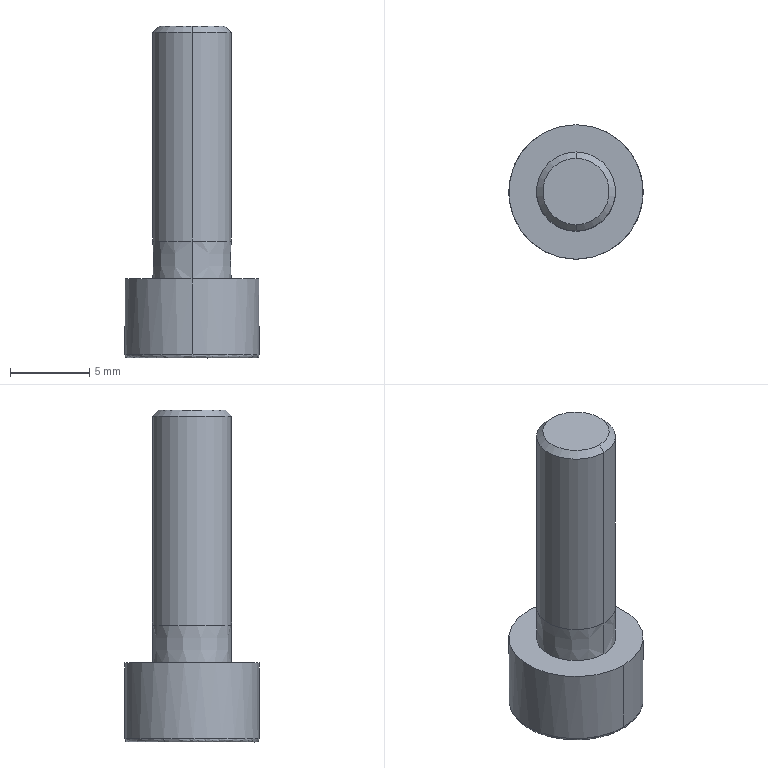Part | SolidWorks | features BaseBody 1 | 1 solid | 20 faces | box 8.5 x 8.5 x 21 mm | volume 561.793 mm3 | plane 10 | cylinder 4 | cone 4 | spline 2 | commonest cylinder face diameters 5 x2 8.5 x2
STEP:
#1=CARTESIAN_POINT('',(554.51,-172.15,205.745));
#2=VERTEX_POINT('',#1);
#3=CARTESIAN_POINT('',(558.371,-178.177,205.745));
#4=VERTEX_POINT('',#3);
#5=CARTESIAN_POINT('',(558.371,-173.927,205.745));
#6=DIRECTION('',(0.000000001,-0.000000003,1.));
#7=DIRECTION('',(0.,-1.,-0.000000003));
#8=AXIS2_PLACEMENT_3D('',#5,#6,#7);
#9=CIRCLE('',#8,4.25);
#10=EDGE_CURVE('',#2,#4,#9,.T.);
#11=ORIENTED_EDGE('',*,*,#10,.F.);
#12=CARTESIAN_POINT('',(554.692,-172.234,205.545));
#13=VERTEX_POINT('',#12);
#14=CARTESIAN_POINT('',(554.692,-172.234,205.745));
#15=DIRECTION('',(-0.4179,-0.9085,-0.000000003));
#16=DIRECTION('',(-0.9085,0.4179,0.000000002));
#17=AXIS2_PLACEMENT_3D('',#14,#15,#16);
#18=CIRCLE('',#17,0.2);
#19=EDGE_CURVE('',#2,#13,#18,.T.);
#20=ORIENTED_EDGE('',*,*,#19,.T.);
#21=CARTESIAN_POINT('',(562.05,-175.619,205.545));
#22=VERTEX_POINT('',#21);
#23=CARTESIAN_POINT('',(554.692,-172.234,205.545));
#24=CARTESIAN_POINT('',(551.306,-179.593,205.545));
#25=CARTESIAN_POINT('',(558.665,-182.978,205.545));
#26=CARTESIAN_POINT('',(562.05,-175.619,205.545));
#27=(BOUNDED_CURVE()B_SPLINE_CURVE(3,(#23,#24,#25,#26),.UNSPECIFIED.,.F.,.F.)B_SPLINE_CURVE_WITH_KNOTS((4,4),(0.,1.),.UNSPECIFIED.)CURVE()GEOMETRIC_REPRESENTATION_ITEM()RATIONAL_B_SPLINE_CURVE((1.,0.3333,0.3333,1.))REPRESENTATION_ITEM(''));
#28=EDGE_CURVE('',#13,#22,#27,.T.);
#29=ORIENTED_EDGE('',*,*,#28,.T.);
#30=CARTESIAN_POINT('',(562.232,-175.703,205.745));
#31=VERTEX_POINT('',#30);
#32=CARTESIAN_POINT('',(562.05,-175.619,205.745));
#33=DIRECTION('',(0.4179,0.9085,0.000000003));
#34=DIRECTION('',(0.9085,-0.4179,-0.000000002));
#35=AXIS2_PLACEMENT_3D('',#32,#33,#34);
#36=CIRCLE('',#35,0.2);
#37=EDGE_CURVE('',#31,#22,#36,.T.);
#38=ORIENTED_EDGE('',*,*,#37,.F.);
#39=CARTESIAN_POINT('',(558.371,-173.927,205.745));
#40=DIRECTION('',(0.000000001,-0.000000003,1.));
#41=DIRECTION('',(0.,-1.,-0.000000003));
#42=AXIS2_PLACEMENT_3D('',#39,#40,#41);
#43=CIRCLE('',#42,4.25);
#44=EDGE_CURVE('',#4,#31,#43,.T.);
#45=ORIENTED_EDGE('',*,*,#44,.F.);
#46=EDGE_LOOP('',(#11,#20,#29,#38,#45));
#47=FACE_OUTER_BOUND('',#46,.T.);
#48=CARTESIAN_POINT('',(554.51,-172.15,205.745));
#49=CARTESIAN_POINT('',(550.957,-179.872,205.745));
#50=CARTESIAN_POINT('',(558.68,-183.425,205.745));
#51=CARTESIAN_POINT('',(562.232,-175.703,205.745));
#52=CARTESIAN_POINT('',(554.51,-172.15,205.627));
#53=CARTESIAN_POINT('',(550.957,-179.872,205.627));
#54=CARTESIAN_POINT('',(558.68,-183.425,205.627));
#55=CARTESIAN_POINT('',(562.232,-175.703,205.627));
#56=CARTESIAN_POINT('',(554.585,-172.185,205.545));
#57=CARTESIAN_POINT('',(551.102,-179.756,205.545));
#58=CARTESIAN_POINT('',(558.674,-183.24,205.545));
#59=CARTESIAN_POINT('',(562.157,-175.668,205.545));
#60=CARTESIAN_POINT('',(554.692,-172.234,205.545));
#61=CARTESIAN_POINT('',(551.306,-179.593,205.545));
#62=CARTESIAN_POINT('',(558.665,-182.978,205.545));
#63=CARTESIAN_POINT('',(562.05,-175.619,205.545));
#64=(BOUNDED_SURFACE()B_SPLINE_SURFACE(3,3,((#48,#49,#50,#51),(#52,#53,#54,#55),(#56,#57,#58,#59),(#60,#61,#62,#63)),.UNSPECIFIED.,.F.,.F.,.F.)B_SPLINE_SURFACE_WITH_KNOTS((4,4),(4,4),(0.,1.),(0.,1.),.UNSPECIFIED.)GEOMETRIC_REPRESENTATION_ITEM()RATIONAL_B_SPLINE_SURFACE(((1.,0.3333,0.3333,1.),(0.8047,0.2682,0.2682,0.8047),(0.8047,0.2682,0.2682,0.8047),(1.,0.3333,0.3333,1.)))REPRESENTATION_ITEM('')SURFACE());
#65=ADVANCED_FACE('',(#47),#64,.T.);
#66=CARTESIAN_POINT('',(558.371,-176.427,212.945));
#67=VERTEX_POINT('',#66);
#68=CARTESIAN_POINT('',(558.371,-171.427,212.945));
#69=VERTEX_POINT('',#68);
#70=CARTESIAN_POINT('',(558.371,-173.927,212.945));
#71=DIRECTION('',(0.000000001,-0.000000003,1.));
#72=DIRECTION('',(0.,-1.,-0.000000003));
#73=AXIS2_PLACEMENT_3D('',#70,#71,#72);
#74=CIRCLE('',#73,2.5);
#75=EDGE_CURVE('',#67,#69,#74,.T.);
#76=ORIENTED_EDGE('',*,*,#75,.T.);
#77=CARTESIAN_POINT('',(558.371,-171.427,226.145));
#78=VERTEX_POINT('',#77);
#79=CARTESIAN_POINT('',(558.371,-171.427,219.545));
#80=DIRECTION('',(0.000000001,-0.000000003,1.));
#81=VECTOR('',#80,1000.);
#82=LINE('',#79,#81);
#83=EDGE_CURVE('',#69,#78,#82,.T.);
#84=ORIENTED_EDGE('',*,*,#83,.T.);
#85=CARTESIAN_POINT('',(558.371,-176.427,226.145));
#86=VERTEX_POINT('',#85);
#87=CARTESIAN_POINT('',(558.371,-173.927,226.145));
#88=DIRECTION('',(-0.000000001,0.000000003,-1.));
#89=DIRECTION('',(0.,-1.,-0.000000003));
#90=AXIS2_PLACEMENT_3D('',#87,#88,#89);
#91=CIRCLE('',#90,2.5);
#92=EDGE_CURVE('',#78,#86,#91,.T.);
#93=ORIENTED_EDGE('',*,*,#92,.T.);
#94=CARTESIAN_POINT('',(558.371,-176.427,219.545));
#95=DIRECTION('',(0.000000001,-0.000000003,1.));
#96=VECTOR('',#95,1000.);
#97=LINE('',#94,#96);
#98=EDGE_CURVE('',#67,#86,#97,.T.);
#99=ORIENTED_EDGE('',*,*,#98,.F.);
#100=EDGE_LOOP('',(#76,#84,#93,#99));
#101=FACE_OUTER_BOUND('',#100,.T.);
#102=CARTESIAN_POINT('',(558.371,-173.927,219.545));
#103=DIRECTION('',(0.000000001,-0.000000003,1.));
#104=DIRECTION('',(0.,-1.,-0.000000003));
#105=AXIS2_PLACEMENT_3D('',#102,#103,#104);
#106=CYLINDRICAL_SURFACE('',#105,2.5);
#107=ADVANCED_FACE('',(#101),#106,.T.);
#108=CARTESIAN_POINT('',(558.371,-171.827,226.545));
#109=VERTEX_POINT('',#108);
#110=CARTESIAN_POINT('',(558.371,-176.027,226.545));
#111=VERTEX_POINT('',#110);
#112=CARTESIAN_POINT('',(558.371,-173.927,226.545));
#113=DIRECTION('',(-0.000000001,0.000000003,-1.));
#114=DIRECTION('',(0.,1.,0.000000003));
#115=AXIS2_PLACEMENT_3D('',#112,#113,#114);
#116=CIRCLE('',#115,2.1);
#117=EDGE_CURVE('',#109,#111,#116,.T.);
#118=ORIENTED_EDGE('',*,*,#117,.T.);
#119=CARTESIAN_POINT('',(558.371,-176.427,226.145));
#120=DIRECTION('',(-0.000000001,-0.7071,-0.7071));
#121=VECTOR('',#120,1000.);
#122=LINE('',#119,#121);
#123=EDGE_CURVE('',#111,#86,#122,.T.);
#124=ORIENTED_EDGE('',*,*,#123,.T.);
#125=ORIENTED_EDGE('',*,*,#92,.F.);
#126=CARTESIAN_POINT('',(558.371,-171.427,226.145));
#127=DIRECTION('',(-0.000000001,0.7071,-0.7071));
#128=VECTOR('',#127,1000.);
#129=LINE('',#126,#128);
#130=EDGE_CURVE('',#109,#78,#129,.T.);
#131=ORIENTED_EDGE('',*,*,#130,.F.);
#132=EDGE_LOOP('',(#118,#124,#125,#131));
#133=FACE_OUTER_BOUND('',#132,.T.);
#134=CARTESIAN_POINT('',(558.371,-173.927,226.145));
#135=DIRECTION('',(-0.000000001,0.000000003,-1.));
#136=DIRECTION('',(0.,1.,0.000000003));
#137=AXIS2_PLACEMENT_3D('',#134,#135,#136);
#138=CONICAL_SURFACE('',#137,2.5,0.7854);
#139=ADVANCED_FACE('',(#133),#138,.T.);
#140=CARTESIAN_POINT('',(558.371,-176.425,210.545));
#141=VERTEX_POINT('',#140);
#142=CARTESIAN_POINT('',(558.371,-171.428,210.545));
#143=VERTEX_POINT('',#142);
#144=CARTESIAN_POINT('',(558.371,-173.927,210.545));
#145=DIRECTION('',(0.000000001,-0.000000003,1.));
#146=DIRECTION('',(0.,-1.,-0.000000003));
#147=AXIS2_PLACEMENT_3D('',#144,#145,#146);
#148=CIRCLE('',#147,2.499);
#149=EDGE_CURVE('',#141,#143,#148,.T.);
#150=ORIENTED_EDGE('',*,*,#149,.T.);
#151=CARTESIAN_POINT('',(558.371,-171.427,212.945));
#152=DIRECTION('',(0.000000001,0.0005208,1.));
#153=VECTOR('',#152,1000.);
#154=LINE('',#151,#153);
#155=EDGE_CURVE('',#143,#69,#154,.T.);
#156=ORIENTED_EDGE('',*,*,#155,.T.);
#157=ORIENTED_EDGE('',*,*,#75,.F.);
#158=CARTESIAN_POINT('',(558.371,-176.427,212.945));
#159=DIRECTION('',(0.000000001,-0.0005208,1.));
#160=VECTOR('',#159,1000.);
#161=LINE('',#158,#160);
#162=EDGE_CURVE('',#141,#67,#161,.T.);
#163=ORIENTED_EDGE('',*,*,#162,.F.);
#164=EDGE_LOOP('',(#150,#156,#157,#163));
#165=FACE_OUTER_BOUND('',#164,.T.);
#166=CARTESIAN_POINT('',(558.371,-173.927,212.945));
#167=DIRECTION('',(0.000000001,-0.000000003,1.));
#168=DIRECTION('',(0.,-1.,-0.000000003));
#169=AXIS2_PLACEMENT_3D('',#166,#167,#168);
#170=CONICAL_SURFACE('',#169,2.5,0.0005208);
#171=ADVANCED_FACE('',(#165),#170,.T.);
#172=ORIENTED_EDGE('',*,*,#44,.T.);
#173=CARTESIAN_POINT('',(558.371,-169.677,205.745));
#174=VERTEX_POINT('',#173);
#175=CARTESIAN_POINT('',(558.371,-173.927,205.745));
#176=DIRECTION('',(0.000000001,-0.000000003,1.));
#177=DIRECTION('',(0.,-1.,-0.000000003));
#178=AXIS2_PLACEMENT_3D('',#175,#176,#177);
#179=CIRCLE('',#178,4.25);
#180=EDGE_CURVE('',#31,#174,#179,.T.);
#181=ORIENTED_EDGE('',*,*,#180,.T.);
#182=CARTESIAN_POINT('',(558.371,-169.677,210.545));
#183=VERTEX_POINT('',#182);
#184=CARTESIAN_POINT('',(558.371,-169.677,208.145));
#185=DIRECTION('',(0.000000001,-0.000000003,1.));
#186=VECTOR('',#185,1000.);
#187=LINE('',#184,#186);
#188=EDGE_CURVE('',#174,#183,#187,.T.);
#189=ORIENTED_EDGE('',*,*,#188,.T.);
#190=CARTESIAN_POINT('',(558.371,-178.177,210.545));
#191=VERTEX_POINT('',#190);
#192=CARTESIAN_POINT('',(558.371,-173.927,210.545));
#193=DIRECTION('',(0.000000001,-0.000000003,1.));
#194=DIRECTION('',(0.,-1.,-0.000000003));
#195=AXIS2_PLACEMENT_3D('',#192,#193,#194);
#196=CIRCLE('',#195,4.25);
#197=EDGE_CURVE('',#191,#183,#196,.T.);
#198=ORIENTED_EDGE('',*,*,#197,.F.);
#199=CARTESIAN_POINT('',(558.371,-178.177,208.145));
#200=DIRECTION('',(0.000000001,-0.000000003,1.));
#201=VECTOR('',#200,1000.);
#202=LINE('',#199,#201);
#203=EDGE_CURVE('',#4,#191,#202,.T.);
#204=ORIENTED_EDGE('',*,*,#203,.F.);
#205=EDGE_LOOP('',(#172,#181,#189,#198,#204));
#206=FACE_OUTER_BOUND('',#205,.T.);
#207=CARTESIAN_POINT('',(558.371,-173.927,208.145));
#208=DIRECTION('',(0.000000001,-0.000000003,1.));
#209=DIRECTION('',(0.,-1.,-0.000000003));
#210=AXIS2_PLACEMENT_3D('',#207,#208,#209);
#211=CYLINDRICAL_SURFACE('',#210,4.25);
#212=ADVANCED_FACE('',(#206),#211,.T.);
#213=ORIENTED_EDGE('',*,*,#83,.F.);
#214=CARTESIAN_POINT('',(558.371,-173.927,212.945));
#215=DIRECTION('',(0.000000001,-0.000000003,1.));
#216=DIRECTION('',(0.,-1.,-0.000000003));
#217=AXIS2_PLACEMENT_3D('',#214,#215,#216);
#218=CIRCLE('',#217,2.5);
#219=EDGE_CURVE('',#69,#67,#218,.T.);
#220=ORIENTED_EDGE('',*,*,#219,.T.);
#221=ORIENTED_EDGE('',*,*,#98,.T.);
#222=CARTESIAN_POINT('',(558.371,-173.927,226.145));
#223=DIRECTION('',(-0.000000001,0.000000003,-1.));
#224=DIRECTION('',(0.,-1.,-0.000000003));
#225=AXIS2_PLACEMENT_3D('',#222,#223,#224);
#226=CIRCLE('',#225,2.5);
#227=EDGE_CURVE('',#86,#78,#226,.T.);
#228=ORIENTED_EDGE('',*,*,#227,.T.);
#229=EDGE_LOOP('',(#213,#220,#221,#228));
#230=FACE_OUTER_BOUND('',#229,.T.);
#231=CARTESIAN_POINT('',(558.371,-173.927,219.545));
#232=DIRECTION('',(0.000000001,-0.000000003,1.));
#233=DIRECTION('',(0.,-1.,-0.000000003));
#234=AXIS2_PLACEMENT_3D('',#231,#232,#233);
#235=CYLINDRICAL_SURFACE('',#234,2.5);
#236=ADVANCED_FACE('',(#230),#235,.T.);
#237=ORIENTED_EDGE('',*,*,#123,.F.);
#238=CARTESIAN_POINT('',(558.371,-173.927,226.545));
#239=DIRECTION('',(-0.000000001,0.000000003,-1.));
#240=DIRECTION('',(0.,1.,0.000000003));
#241=AXIS2_PLACEMENT_3D('',#238,#239,#240);
#242=CIRCLE('',#241,2.1);
#243=EDGE_CURVE('',#111,#109,#242,.T.);
#244=ORIENTED_EDGE('',*,*,#243,.T.);
#245=ORIENTED_EDGE('',*,*,#130,.T.);
#246=ORIENTED_EDGE('',*,*,#227,.F.);
#247=EDGE_LOOP('',(#237,#244,#245,#246));
#248=FACE_OUTER_BOUND('',#247,.T.);
#249=CARTESIAN_POINT('',(558.371,-173.927,226.145));
#250=DIRECTION('',(-0.000000001,0.000000003,-1.));
#251=DIRECTION('',(0.,1.,0.000000003));
#252=AXIS2_PLACEMENT_3D('',#249,#250,#251);
#253=CONICAL_SURFACE('',#252,2.5,0.7854);
#254=ADVANCED_FACE('',(#248),#253,.T.);
#255=ORIENTED_EDGE('',*,*,#155,.F.);
#256=CARTESIAN_POINT('',(558.371,-173.927,210.545));
#257=DIRECTION('',(0.000000001,-0.000000003,1.));
#258=DIRECTION('',(0.,-1.,-0.000000003));
#259=AXIS2_PLACEMENT_3D('',#256,#257,#258);
#260=CIRCLE('',#259,2.499);
#261=EDGE_CURVE('',#143,#141,#260,.T.);
#262=ORIENTED_EDGE('',*,*,#261,.T.);
#263=ORIENTED_EDGE('',*,*,#162,.T.);
#264=ORIENTED_EDGE('',*,*,#219,.F.);
#265=EDGE_LOOP('',(#255,#262,#263,#264));
#266=FACE_OUTER_BOUND('',#265,.T.);
#267=CARTESIAN_POINT('',(558.371,-173.927,212.945));
#268=DIRECTION('',(0.000000001,-0.000000003,1.));
#269=DIRECTION('',(0.,-1.,-0.000000003));
#270=AXIS2_PLACEMENT_3D('',#267,#268,#269);
#271=CONICAL_SURFACE('',#270,2.5,0.0005208);
#272=ADVANCED_FACE('',(#266),#271,.T.);
#273=ORIENTED_EDGE('',*,*,#117,.F.);
#274=ORIENTED_EDGE('',*,*,#243,.F.);
#275=EDGE_LOOP('',(#273,#274));
#276=FACE_OUTER_BOUND('',#275,.T.);
#277=CARTESIAN_POINT('',(559.325,-174.365,226.545));
#278=DIRECTION('',(0.000000001,-0.000000003,1.));
#279=DIRECTION('',(0.,-1.,-0.000000003));
#280=AXIS2_PLACEMENT_3D('',#277,#278,#279);
#281=PLANE('',#280);
#282=ADVANCED_FACE('',(#276),#281,.T.);
#283=ORIENTED_EDGE('',*,*,#149,.F.);
#284=ORIENTED_EDGE('',*,*,#261,.F.);
#285=EDGE_LOOP('',(#283,#284));
#286=FACE_BOUND('',#285,.T.);
#287=ORIENTED_EDGE('',*,*,#197,.T.);
#288=CARTESIAN_POINT('',(558.371,-173.927,210.545));
#289=DIRECTION('',(0.000000001,-0.000000003,1.));
#290=DIRECTION('',(0.,-1.,-0.000000003));
#291=AXIS2_PLACEMENT_3D('',#288,#289,#290);
#292=CIRCLE('',#291,4.25);
#293=EDGE_CURVE('',#183,#191,#292,.T.);
#294=ORIENTED_EDGE('',*,*,#293,.T.);
#295=EDGE_LOOP('',(#287,#294));
#296=FACE_OUTER_BOUND('',#295,.T.);
#297=CARTESIAN_POINT('',(560.302,-174.815,210.545));
#298=DIRECTION('',(0.000000001,-0.000000003,1.));
#299=DIRECTION('',(0.,-1.,-0.000000003));
#300=AXIS2_PLACEMENT_3D('',#297,#298,#299);
#301=PLANE('',#300);
#302=ADVANCED_FACE('',(#286,#296),#301,.T.);
#303=ORIENTED_EDGE('',*,*,#188,.F.);
#304=CARTESIAN_POINT('',(558.371,-173.927,205.745));
#305=DIRECTION('',(0.000000001,-0.000000003,1.));
#306=DIRECTION('',(0.,-1.,-0.000000003));
#307=AXIS2_PLACEMENT_3D('',#304,#305,#306);
#308=CIRCLE('',#307,4.25);
#309=EDGE_CURVE('',#174,#2,#308,.T.);
#310=ORIENTED_EDGE('',*,*,#309,.T.);
#311=ORIENTED_EDGE('',*,*,#10,.T.);
#312=ORIENTED_EDGE('',*,*,#203,.T.);
#313=ORIENTED_EDGE('',*,*,#293,.F.);
#314=EDGE_LOOP('',(#303,#310,#311,#312,#313));
#315=FACE_OUTER_BOUND('',#314,.T.);
#316=CARTESIAN_POINT('',(558.371,-173.927,208.145));
#317=DIRECTION('',(0.000000001,-0.000000003,1.));
#318=DIRECTION('',(0.,-1.,-0.000000003));
#319=AXIS2_PLACEMENT_3D('',#316,#317,#318);
#320=CYLINDRICAL_SURFACE('',#319,4.25);
#321=ADVANCED_FACE('',(#315),#320,.T.);
#322=ORIENTED_EDGE('',*,*,#19,.F.);
#323=ORIENTED_EDGE('',*,*,#309,.F.);
#324=ORIENTED_EDGE('',*,*,#180,.F.);
#325=ORIENTED_EDGE('',*,*,#37,.T.);
#326=CARTESIAN_POINT('',(562.05,-175.619,205.545));
#327=CARTESIAN_POINT('',(565.436,-168.261,205.545));
#328=CARTESIAN_POINT('',(558.077,-164.875,205.545));
#329=CARTESIAN_POINT('',(554.692,-172.234,205.545));
#330=(BOUNDED_CURVE()B_SPLINE_CURVE(3,(#326,#327,#328,#329),.UNSPECIFIED.,.F.,.F.)B_SPLINE_CURVE_WITH_KNOTS((4,4),(0.,1.),.UNSPECIFIED.)CURVE()GEOMETRIC_REPRESENTATION_ITEM()RATIONAL_B_SPLINE_CURVE((1.,0.3333,0.3333,1.))REPRESENTATION_ITEM(''));
#331=EDGE_CURVE('',#22,#13,#330,.T.);
#332=ORIENTED_EDGE('',*,*,#331,.T.);
#333=EDGE_LOOP('',(#322,#323,#324,#325,#332));
#334=FACE_OUTER_BOUND('',#333,.T.);
#335=CARTESIAN_POINT('',(562.232,-175.703,205.745));
#336=CARTESIAN_POINT('',(565.785,-167.981,205.745));
#337=CARTESIAN_POINT('',(558.062,-164.428,205.745));
#338=CARTESIAN_POINT('',(554.51,-172.15,205.745));
#339=CARTESIAN_POINT('',(562.232,-175.703,205.627));
#340=CARTESIAN_POINT('',(565.785,-167.981,205.627));
#341=CARTESIAN_POINT('',(558.062,-164.428,205.627));
#342=CARTESIAN_POINT('',(554.51,-172.15,205.627));
#343=CARTESIAN_POINT('',(562.157,-175.668,205.545));
#344=CARTESIAN_POINT('',(565.64,-168.097,205.545));
#345=CARTESIAN_POINT('',(558.068,-164.613,205.545));
#346=CARTESIAN_POINT('',(554.585,-172.185,205.545));
#347=CARTESIAN_POINT('',(562.05,-175.619,205.545));
#348=CARTESIAN_POINT('',(565.436,-168.261,205.545));
#349=CARTESIAN_POINT('',(558.077,-164.875,205.545));
#350=CARTESIAN_POINT('',(554.692,-172.234,205.545));
#351=(BOUNDED_SURFACE()B_SPLINE_SURFACE(3,3,((#335,#336,#337,#338),(#339,#340,#341,#342),(#343,#344,#345,#346),(#347,#348,#349,#350)),.UNSPECIFIED.,.F.,.F.,.F.)B_SPLINE_SURFACE_WITH_KNOTS((4,4),(4,4),(0.,1.),(0.,1.),.UNSPECIFIED.)GEOMETRIC_REPRESENTATION_ITEM()RATIONAL_B_SPLINE_SURFACE(((1.,0.3333,0.3333,1.),(0.8047,0.2682,0.2682,0.8047),(0.8047,0.2682,0.2682,0.8047),(1.,0.3333,0.3333,1.)))REPRESENTATION_ITEM('')SURFACE());
#352=ADVANCED_FACE('',(#334),#351,.T.);
#353=ORIENTED_EDGE('',*,*,#28,.F.);
#354=ORIENTED_EDGE('',*,*,#331,.F.);
#355=EDGE_LOOP('',(#353,#354));
#356=FACE_OUTER_BOUND('',#355,.T.);
#357=CARTESIAN_POINT('',(558.158,-171.627,205.545));
#358=VERTEX_POINT('',#357);
#359=CARTESIAN_POINT('',(556.273,-172.961,205.545));
#360=VERTEX_POINT('',#359);
#361=CARTESIAN_POINT('',(558.158,-171.627,205.545));
#362=DIRECTION('',(-0.8162,-0.5778,-0.000000001));
#363=VECTOR('',#362,1000.);
#364=LINE('',#361,#363);
#365=EDGE_CURVE('',#358,#360,#364,.T.);
#366=ORIENTED_EDGE('',*,*,#365,.T.);
#367=CARTESIAN_POINT('',(556.486,-175.261,205.545));
#368=VERTEX_POINT('',#367);
#369=CARTESIAN_POINT('',(556.273,-172.961,205.545));
#370=DIRECTION('',(0.09229,-0.9957,-0.000000003));
#371=VECTOR('',#370,1000.);
#372=LINE('',#369,#371);
#373=EDGE_CURVE('',#360,#368,#372,.T.);
#374=ORIENTED_EDGE('',*,*,#373,.T.);
#375=CARTESIAN_POINT('',(558.584,-176.226,205.545));
#376=VERTEX_POINT('',#375);
#377=CARTESIAN_POINT('',(556.486,-175.261,205.545));
#378=DIRECTION('',(0.9085,-0.4179,-0.000000002));
#379=VECTOR('',#378,1000.);
#380=LINE('',#377,#379);
#381=EDGE_CURVE('',#368,#376,#380,.T.);
#382=ORIENTED_EDGE('',*,*,#381,.T.);
#383=CARTESIAN_POINT('',(560.469,-174.892,205.545));
#384=VERTEX_POINT('',#383);
#385=CARTESIAN_POINT('',(558.584,-176.226,205.545));
#386=DIRECTION('',(0.8162,0.5778,0.000000001));
#387=VECTOR('',#386,1000.);
#388=LINE('',#385,#387);
#389=EDGE_CURVE('',#376,#384,#388,.T.);
#390=ORIENTED_EDGE('',*,*,#389,.T.);
#391=CARTESIAN_POINT('',(560.256,-172.592,205.545));
#392=VERTEX_POINT('',#391);
#393=CARTESIAN_POINT('',(560.469,-174.892,205.545));
#394=DIRECTION('',(-0.09229,0.9957,0.000000003));
#395=VECTOR('',#394,1000.);
#396=LINE('',#393,#395);
#397=EDGE_CURVE('',#384,#392,#396,.T.);
#398=ORIENTED_EDGE('',*,*,#397,.T.);
#399=CARTESIAN_POINT('',(560.256,-172.592,205.545));
#400=DIRECTION('',(-0.9085,0.4179,0.000000002));
#401=VECTOR('',#400,1000.);
#402=LINE('',#399,#401);
#403=EDGE_CURVE('',#392,#358,#402,.T.);
#404=ORIENTED_EDGE('',*,*,#403,.T.);
#405=EDGE_LOOP('',(#366,#374,#382,#390,#398,#404));
#406=FACE_BOUND('',#405,.T.);
#407=CARTESIAN_POINT('',(560.211,-174.773,205.545));
#408=DIRECTION('',(-0.000000001,0.000000003,-1.));
#409=DIRECTION('',(0.,1.,0.000000003));
#410=AXIS2_PLACEMENT_3D('',#407,#408,#409);
#411=PLANE('',#410);
#412=ADVANCED_FACE('',(#356,#406),#411,.T.);
#413=CARTESIAN_POINT('',(556.486,-175.261,208.045));
#414=VERTEX_POINT('',#413);
#415=CARTESIAN_POINT('',(556.486,-175.261,205.545));
#416=DIRECTION('',(0.,0.,1.));
#417=VECTOR('',#416,1000.);
#418=LINE('',#415,#417);
#419=EDGE_CURVE('',#368,#414,#418,.T.);
#420=ORIENTED_EDGE('',*,*,#419,.F.);
#421=ORIENTED_EDGE('',*,*,#373,.F.);
#422=CARTESIAN_POINT('',(556.273,-172.961,208.045));
#423=VERTEX_POINT('',#422);
#424=CARTESIAN_POINT('',(556.273,-172.961,205.545));
#425=DIRECTION('',(0.,0.,-1.));
#426=VECTOR('',#425,1000.);
#427=LINE('',#424,#426);
#428=EDGE_CURVE('',#423,#360,#427,.T.);
#429=ORIENTED_EDGE('',*,*,#428,.F.);
#430=CARTESIAN_POINT('',(556.486,-175.261,208.045));
#431=DIRECTION('',(-0.09229,0.9957,0.));
#432=VECTOR('',#431,1000.);
#433=LINE('',#430,#432);
#434=EDGE_CURVE('',#414,#423,#433,.T.);
#435=ORIENTED_EDGE('',*,*,#434,.F.);
#436=EDGE_LOOP('',(#420,#421,#429,#435));
#437=FACE_OUTER_BOUND('',#436,.T.);
#438=CARTESIAN_POINT('',(556.486,-175.261,205.545));
#439=DIRECTION('',(-0.9957,-0.09229,0.));
#440=DIRECTION('',(0.09229,-0.9957,0.));
#441=AXIS2_PLACEMENT_3D('',#438,#439,#440);
#442=PLANE('',#441);
#443=ADVANCED_FACE('',(#437),#442,.F.);
#444=ORIENTED_EDGE('',*,*,#428,.T.);
#445=ORIENTED_EDGE('',*,*,#365,.F.);
#446=CARTESIAN_POINT('',(558.158,-171.627,208.045));
#447=VERTEX_POINT('',#446);
#448=CARTESIAN_POINT('',(558.158,-171.627,205.545));
#449=DIRECTION('',(-0.000000002,0.000000003,-1.));
#450=VECTOR('',#449,1000.);
#451=LINE('',#448,#450);
#452=EDGE_CURVE('',#447,#358,#451,.T.);
#453=ORIENTED_EDGE('',*,*,#452,.F.);
#454=CARTESIAN_POINT('',(556.273,-172.961,208.045));
#455=DIRECTION('',(0.8162,0.5778,0.));
#456=VECTOR('',#455,1000.);
#457=LINE('',#454,#456);
#458=EDGE_CURVE('',#423,#447,#457,.T.);
#459=ORIENTED_EDGE('',*,*,#458,.F.);
#460=EDGE_LOOP('',(#444,#445,#453,#459));
#461=FACE_OUTER_BOUND('',#460,.T.);
#462=CARTESIAN_POINT('',(556.273,-172.961,205.545));
#463=DIRECTION('',(-0.5778,0.8162,0.000000003));
#464=DIRECTION('',(-0.8162,-0.5778,0.));
#465=AXIS2_PLACEMENT_3D('',#462,#463,#464);
#466=PLANE('',#465);
#467=ADVANCED_FACE('',(#461),#466,.F.);
#468=ORIENTED_EDGE('',*,*,#452,.T.);
#469=ORIENTED_EDGE('',*,*,#403,.F.);
#470=CARTESIAN_POINT('',(560.256,-172.592,208.045));
#471=VERTEX_POINT('',#470);
#472=CARTESIAN_POINT('',(560.256,-172.592,205.545));
#473=DIRECTION('',(0.000000001,0.000000002,-1.));
#474=VECTOR('',#473,1000.);
#475=LINE('',#472,#474);
#476=EDGE_CURVE('',#471,#392,#475,.T.);
#477=ORIENTED_EDGE('',*,*,#476,.F.);
#478=CARTESIAN_POINT('',(558.158,-171.627,208.045));
#479=DIRECTION('',(0.9085,-0.4179,0.));
#480=VECTOR('',#479,1000.);
#481=LINE('',#478,#480);
#482=EDGE_CURVE('',#447,#471,#481,.T.);
#483=ORIENTED_EDGE('',*,*,#482,.F.);
#484=EDGE_LOOP('',(#468,#469,#477,#483));
#485=FACE_OUTER_BOUND('',#484,.T.);
#486=CARTESIAN_POINT('',(558.158,-171.627,205.545));
#487=DIRECTION('',(0.4179,0.9085,0.000000003));
#488=DIRECTION('',(-0.9085,0.4179,0.));
#489=AXIS2_PLACEMENT_3D('',#486,#487,#488);
#490=PLANE('',#489);
#491=ADVANCED_FACE('',(#485),#490,.F.);
#492=ORIENTED_EDGE('',*,*,#476,.T.);
#493=ORIENTED_EDGE('',*,*,#397,.F.);
#494=CARTESIAN_POINT('',(560.469,-174.892,208.045));
#495=VERTEX_POINT('',#494);
#496=CARTESIAN_POINT('',(560.469,-174.892,205.545));
#497=DIRECTION('',(0.,0.,-1.));
#498=VECTOR('',#497,1000.);
#499=LINE('',#496,#498);
#500=EDGE_CURVE('',#495,#384,#499,.T.);
#501=ORIENTED_EDGE('',*,*,#500,.F.);
#502=CARTESIAN_POINT('',(560.256,-172.592,208.045));
#503=DIRECTION('',(0.09229,-0.9957,0.));
#504=VECTOR('',#503,1000.);
#505=LINE('',#502,#504);
#506=EDGE_CURVE('',#471,#495,#505,.T.);
#507=ORIENTED_EDGE('',*,*,#506,.F.);
#508=EDGE_LOOP('',(#492,#493,#501,#507));
#509=FACE_OUTER_BOUND('',#508,.T.);
#510=CARTESIAN_POINT('',(560.256,-172.592,205.545));
#511=DIRECTION('',(0.9957,0.09229,0.));
#512=DIRECTION('',(-0.09229,0.9957,0.));
#513=AXIS2_PLACEMENT_3D('',#510,#511,#512);
#514=PLANE('',#513);
#515=ADVANCED_FACE('',(#509),#514,.F.);
#516=ORIENTED_EDGE('',*,*,#500,.T.);
#517=ORIENTED_EDGE('',*,*,#389,.F.);
#518=CARTESIAN_POINT('',(558.584,-176.226,208.045));
#519=VERTEX_POINT('',#518);
#520=CARTESIAN_POINT('',(558.584,-176.226,205.545));
#521=DIRECTION('',(-0.000000002,0.000000003,-1.));
#522=VECTOR('',#521,1000.);
#523=LINE('',#520,#522);
#524=EDGE_CURVE('',#519,#376,#523,.T.);
#525=ORIENTED_EDGE('',*,*,#524,.F.);
#526=CARTESIAN_POINT('',(560.469,-174.892,208.045));
#527=DIRECTION('',(-0.8162,-0.5778,0.));
#528=VECTOR('',#527,1000.);
#529=LINE('',#526,#528);
#530=EDGE_CURVE('',#495,#519,#529,.T.);
#531=ORIENTED_EDGE('',*,*,#530,.F.);
#532=EDGE_LOOP('',(#516,#517,#525,#531));
#533=FACE_OUTER_BOUND('',#532,.T.);
#534=CARTESIAN_POINT('',(560.469,-174.892,205.545));
#535=DIRECTION('',(0.5778,-0.8162,-0.000000003));
#536=DIRECTION('',(0.8162,0.5778,0.));
#537=AXIS2_PLACEMENT_3D('',#534,#535,#536);
#538=PLANE('',#537);
#539=ADVANCED_FACE('',(#533),#538,.F.);
#540=ORIENTED_EDGE('',*,*,#524,.T.);
#541=ORIENTED_EDGE('',*,*,#381,.F.);
#542=ORIENTED_EDGE('',*,*,#419,.T.);
#543=CARTESIAN_POINT('',(558.584,-176.226,208.045));
#544=DIRECTION('',(-0.9085,0.4179,0.));
#545=VECTOR('',#544,1000.);
#546=LINE('',#543,#545);
#547=EDGE_CURVE('',#519,#414,#546,.T.);
#548=ORIENTED_EDGE('',*,*,#547,.F.);
#549=EDGE_LOOP('',(#540,#541,#542,#548));
#550=FACE_OUTER_BOUND('',#549,.T.);
#551=CARTESIAN_POINT('',(558.584,-176.226,205.545));
#552=DIRECTION('',(-0.4179,-0.9085,-0.000000003));
#553=DIRECTION('',(0.9085,-0.4179,0.));
#554=AXIS2_PLACEMENT_3D('',#551,#552,#553);
#555=PLANE('',#554);
#556=ADVANCED_FACE('',(#550),#555,.F.);
#557=ORIENTED_EDGE('',*,*,#506,.T.);
#558=ORIENTED_EDGE('',*,*,#530,.T.);
#559=ORIENTED_EDGE('',*,*,#547,.T.);
#560=ORIENTED_EDGE('',*,*,#434,.T.);
#561=ORIENTED_EDGE('',*,*,#458,.T.);
#562=ORIENTED_EDGE('',*,*,#482,.T.);
#563=EDGE_LOOP('',(#557,#558,#559,#560,#561,#562));
#564=FACE_OUTER_BOUND('',#563,.T.);
#565=CARTESIAN_POINT('',(558.371,-173.927,208.045));
#566=DIRECTION('',(-0.000000001,0.000000003,-1.));
#567=DIRECTION('',(0.,1.,0.000000003));
#568=AXIS2_PLACEMENT_3D('',#565,#566,#567);
#569=PLANE('',#568);
#570=ADVANCED_FACE('',(#564),#569,.T.);
#571=CLOSED_SHELL('',(#65,#107,#139,#171,#212,#236,#254,#272,#282,#302,#321,#352,#412,#443,#467,#491,#515,#539,#556,#570));
#572=MANIFOLD_SOLID_BREP('',#571);
#573=CARTESIAN_POINT('',(0.,0.,0.));
#574=DIRECTION('',(0.,0.,1.));
#575=DIRECTION('',(1.,0.,0.));
#576=AXIS2_PLACEMENT_3D('',#573,#574,#575);
#577=(LENGTH_UNIT()NAMED_UNIT(*)SI_UNIT(.MILLI.,.METRE.));
#578=UNCERTAINTY_MEASURE_WITH_UNIT(LENGTH_MEASURE(0.00001),#577,'','');
#579=(NAMED_UNIT(*)PLANE_ANGLE_UNIT()SI_UNIT($,.RADIAN.));
#580=(NAMED_UNIT(*)SI_UNIT($,.STERADIAN.)SOLID_ANGLE_UNIT());
#581=(GEOMETRIC_REPRESENTATION_CONTEXT(3)GLOBAL_UNCERTAINTY_ASSIGNED_CONTEXT((#578))GLOBAL_UNIT_ASSIGNED_CONTEXT((#577,#579,#580))REPRESENTATION_CONTEXT('',''));
#582=ADVANCED_BREP_SHAPE_REPRESENTATION('',(#572,#576),#581);